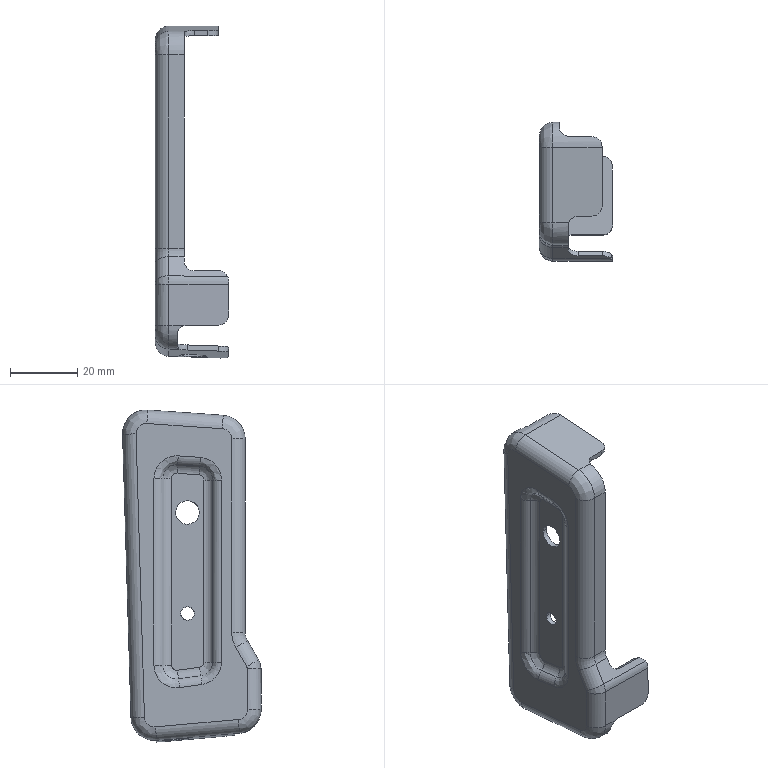Part | 1 solid | 126 faces | box 21.748 x 41.227 x 98.581 mm | volume 8113 mm3 | spline 63 | cylinder 44 | plane 13 | torus 4 | other 2 | commonest cylinder face diameters 6 x8 5 x6 8 x6 3 x4 9 x4 11 x4